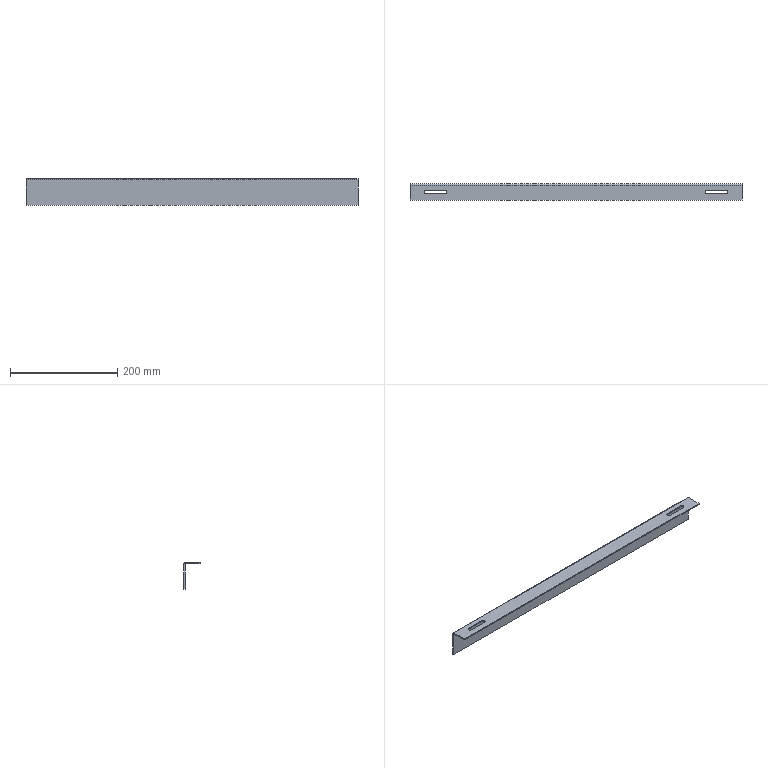Part | STEP file | FHD-021-010 L-shaped support rail | 1 solid | 18 faces | box 620 x 30 x 50 mm | volume 94894 mm3 | plane 12 | cylinder 6 | commonest cylinder face diameters 7 x4 0.6 x1 4.6 x1
STEP:
#1=CARTESIAN_POINT('',(0.,0.,0.));
#2=DIRECTION('',(0.,0.,1.));
#3=DIRECTION('',(1.,0.,0.));
#4=AXIS2_PLACEMENT_3D('',#1,#2,#3);
#5=CARTESIAN_POINT('',(-310.,13.,-2.3));
#6=VERTEX_POINT('',#5);
#7=CARTESIAN_POINT('',(-310.,13.,-50.));
#8=VERTEX_POINT('',#7);
#9=CARTESIAN_POINT('',(-310.,13.,0.));
#10=DIRECTION('',(0.,0.,-1.));
#11=VECTOR('',#10,1.);
#12=LINE('',#9,#11);
#13=CARTESIAN_POINT('',(0.,13.,0.));
#14=DIRECTION('',(0.,-1.,0.));
#15=DIRECTION('',(0.,0.,-1.));
#16=AXIS2_PLACEMENT_3D('',#13,#14,#15);
#17=PLANE('',#16);
#18=CARTESIAN_POINT('',(0.,-310.));
#19=DIRECTION('',(1.,0.));
#20=VECTOR('',#19,1.);
#21=LINE('',#18,#20);
#22=(GEOMETRIC_REPRESENTATION_CONTEXT(2)PARAMETRIC_REPRESENTATION_CONTEXT()REPRESENTATION_CONTEXT('',''));
#23=DEFINITIONAL_REPRESENTATION('',(#21),#22);
#24=PCURVE('',#17,#23);
#25=CARTESIAN_POINT('',(-310.,15.,-2.));
#26=DIRECTION('',(1.,0.,0.));
#27=DIRECTION('',(0.,0.,-1.));
#28=AXIS2_PLACEMENT_3D('',#25,#26,#27);
#29=PLANE('',#28);
#30=CARTESIAN_POINT('',(-2.,-2.));
#31=DIRECTION('',(1.,0.));
#32=VECTOR('',#31,1.);
#33=LINE('',#30,#32);
#34=(GEOMETRIC_REPRESENTATION_CONTEXT(2)PARAMETRIC_REPRESENTATION_CONTEXT()REPRESENTATION_CONTEXT('',''));
#35=DEFINITIONAL_REPRESENTATION('',(#33),#34);
#36=PCURVE('',#29,#35);
#37=SURFACE_CURVE('',#12,(#24,#36),.PCURVE_S1.);
#38=EDGE_CURVE('',#6,#8,#37,.T.);
#39=ORIENTED_EDGE('',*,*,#38,.T.);
#40=CARTESIAN_POINT('',(310.,13.,-50.));
#41=VERTEX_POINT('',#40);
#42=CARTESIAN_POINT('',(0.,13.,-50.));
#43=DIRECTION('',(1.,0.,0.));
#44=VECTOR('',#43,1.);
#45=LINE('',#42,#44);
#46=CARTESIAN_POINT('',(50.,0.));
#47=DIRECTION('',(0.,1.));
#48=VECTOR('',#47,1.);
#49=LINE('',#46,#48);
#50=(GEOMETRIC_REPRESENTATION_CONTEXT(2)PARAMETRIC_REPRESENTATION_CONTEXT()REPRESENTATION_CONTEXT('',''));
#51=DEFINITIONAL_REPRESENTATION('',(#49),#50);
#52=PCURVE('',#17,#51);
#53=CARTESIAN_POINT('',(-310.,15.,-50.));
#54=DIRECTION('',(0.,0.,1.));
#55=DIRECTION('',(0.,-1.,0.));
#56=AXIS2_PLACEMENT_3D('',#53,#54,#55);
#57=PLANE('',#56);
#58=CARTESIAN_POINT('',(2.,310.));
#59=DIRECTION('',(0.,1.));
#60=VECTOR('',#59,1.);
#61=LINE('',#58,#60);
#62=(GEOMETRIC_REPRESENTATION_CONTEXT(2)PARAMETRIC_REPRESENTATION_CONTEXT()REPRESENTATION_CONTEXT('',''));
#63=DEFINITIONAL_REPRESENTATION('',(#61),#62);
#64=PCURVE('',#57,#63);
#65=SURFACE_CURVE('',#45,(#52,#64),.PCURVE_S1.);
#66=EDGE_CURVE('',#8,#41,#65,.T.);
#67=ORIENTED_EDGE('',*,*,#66,.T.);
#68=CARTESIAN_POINT('',(310.,13.,-2.3));
#69=VERTEX_POINT('',#68);
#70=CARTESIAN_POINT('',(310.,13.,0.));
#71=DIRECTION('',(0.,0.,1.));
#72=VECTOR('',#71,1.);
#73=LINE('',#70,#72);
#74=CARTESIAN_POINT('',(0.,310.));
#75=DIRECTION('',(-1.,0.));
#76=VECTOR('',#75,1.);
#77=LINE('',#74,#76);
#78=(GEOMETRIC_REPRESENTATION_CONTEXT(2)PARAMETRIC_REPRESENTATION_CONTEXT()REPRESENTATION_CONTEXT('',''));
#79=DEFINITIONAL_REPRESENTATION('',(#77),#78);
#80=PCURVE('',#17,#79);
#81=CARTESIAN_POINT('',(310.,15.,-50.));
#82=DIRECTION('',(-1.,0.,0.));
#83=DIRECTION('',(0.,0.,1.));
#84=AXIS2_PLACEMENT_3D('',#81,#82,#83);
#85=PLANE('',#84);
#86=CARTESIAN_POINT('',(50.,-2.));
#87=DIRECTION('',(1.,0.));
#88=VECTOR('',#87,1.);
#89=LINE('',#86,#88);
#90=(GEOMETRIC_REPRESENTATION_CONTEXT(2)PARAMETRIC_REPRESENTATION_CONTEXT()REPRESENTATION_CONTEXT('',''));
#91=DEFINITIONAL_REPRESENTATION('',(#89),#90);
#92=PCURVE('',#85,#91);
#93=SURFACE_CURVE('',#73,(#80,#92),.PCURVE_S1.);
#94=EDGE_CURVE('',#41,#69,#93,.T.);
#95=ORIENTED_EDGE('',*,*,#94,.T.);
#96=CARTESIAN_POINT('',(0.,13.,-2.3));
#97=DIRECTION('',(-1.,0.,0.));
#98=VECTOR('',#97,1.);
#99=LINE('',#96,#98);
#100=CARTESIAN_POINT('',(2.3,0.));
#101=DIRECTION('',(0.,-1.));
#102=VECTOR('',#101,1.);
#103=LINE('',#100,#102);
#104=(GEOMETRIC_REPRESENTATION_CONTEXT(2)PARAMETRIC_REPRESENTATION_CONTEXT()REPRESENTATION_CONTEXT('',''));
#105=DEFINITIONAL_REPRESENTATION('',(#103),#104);
#106=PCURVE('',#17,#105);
#107=CARTESIAN_POINT('',(310.,12.7,-2.3));
#108=DIRECTION('',(1.,0.,0.));
#109=DIRECTION('',(0.,0.,-1.));
#110=AXIS2_PLACEMENT_3D('',#107,#108,#109);
#111=CYLINDRICAL_SURFACE('',#110,0.3);
#112=CARTESIAN_POINT('',(1.571,-310.));
#113=DIRECTION('',(0.,-1.));
#114=VECTOR('',#113,1.);
#115=LINE('',#112,#114);
#116=(GEOMETRIC_REPRESENTATION_CONTEXT(2)PARAMETRIC_REPRESENTATION_CONTEXT()REPRESENTATION_CONTEXT('',''));
#117=DEFINITIONAL_REPRESENTATION('',(#115),#116);
#118=PCURVE('',#111,#117);
#119=SURFACE_CURVE('',#99,(#106,#118),.PCURVE_S1.);
#120=EDGE_CURVE('',#69,#6,#119,.T.);
#121=ORIENTED_EDGE('',*,*,#120,.T.);
#122=EDGE_LOOP('',(#39,#67,#95,#121));
#123=FACE_BOUND('',#122,.T.);
#124=ADVANCED_FACE('',(#123),#17,.T.);
#125=CARTESIAN_POINT('',(-310.,15.,-50.));
#126=VERTEX_POINT('',#125);
#127=CARTESIAN_POINT('',(-310.,15.,-50.));
#128=DIRECTION('',(0.,-1.,0.));
#129=VECTOR('',#128,1.);
#130=LINE('',#127,#129);
#131=CARTESIAN_POINT('',(0.,0.));
#132=DIRECTION('',(1.,0.));
#133=VECTOR('',#132,1.);
#134=LINE('',#131,#133);
#135=(GEOMETRIC_REPRESENTATION_CONTEXT(2)PARAMETRIC_REPRESENTATION_CONTEXT()REPRESENTATION_CONTEXT('',''));
#136=DEFINITIONAL_REPRESENTATION('',(#134),#135);
#137=PCURVE('',#57,#136);
#138=CARTESIAN_POINT('',(48.,0.));
#139=DIRECTION('',(0.,-1.));
#140=VECTOR('',#139,1.);
#141=LINE('',#138,#140);
#142=(GEOMETRIC_REPRESENTATION_CONTEXT(2)PARAMETRIC_REPRESENTATION_CONTEXT()REPRESENTATION_CONTEXT('',''));
#143=DEFINITIONAL_REPRESENTATION('',(#141),#142);
#144=PCURVE('',#29,#143);
#145=SURFACE_CURVE('',#130,(#137,#144),.PCURVE_S1.);
#146=EDGE_CURVE('',#126,#8,#145,.T.);
#147=ORIENTED_EDGE('',*,*,#146,.F.);
#148=CARTESIAN_POINT('',(310.,15.,-50.));
#149=VERTEX_POINT('',#148);
#150=CARTESIAN_POINT('',(-310.,15.,-50.));
#151=DIRECTION('',(-1.,0.,0.));
#152=VECTOR('',#151,1.);
#153=LINE('',#150,#152);
#154=CARTESIAN_POINT('',(0.,0.));
#155=DIRECTION('',(0.,-1.));
#156=VECTOR('',#155,1.);
#157=LINE('',#154,#156);
#158=(GEOMETRIC_REPRESENTATION_CONTEXT(2)PARAMETRIC_REPRESENTATION_CONTEXT()REPRESENTATION_CONTEXT('',''));
#159=DEFINITIONAL_REPRESENTATION('',(#157),#158);
#160=PCURVE('',#57,#159);
#161=CARTESIAN_POINT('',(0.,15.,0.));
#162=DIRECTION('',(0.,-1.,0.));
#163=DIRECTION('',(0.,0.,-1.));
#164=AXIS2_PLACEMENT_3D('',#161,#162,#163);
#165=PLANE('',#164);
#166=CARTESIAN_POINT('',(50.,-310.));
#167=DIRECTION('',(0.,-1.));
#168=VECTOR('',#167,1.);
#169=LINE('',#166,#168);
#170=(GEOMETRIC_REPRESENTATION_CONTEXT(2)PARAMETRIC_REPRESENTATION_CONTEXT()REPRESENTATION_CONTEXT('',''));
#171=DEFINITIONAL_REPRESENTATION('',(#169),#170);
#172=PCURVE('',#165,#171);
#173=SURFACE_CURVE('',#153,(#160,#172),.PCURVE_S1.);
#174=EDGE_CURVE('',#149,#126,#173,.T.);
#175=ORIENTED_EDGE('',*,*,#174,.F.);
#176=CARTESIAN_POINT('',(310.,15.,-50.));
#177=DIRECTION('',(0.,1.,0.));
#178=VECTOR('',#177,1.);
#179=LINE('',#176,#178);
#180=CARTESIAN_POINT('',(0.,620.));
#181=DIRECTION('',(-1.,0.));
#182=VECTOR('',#181,1.);
#183=LINE('',#180,#182);
#184=(GEOMETRIC_REPRESENTATION_CONTEXT(2)PARAMETRIC_REPRESENTATION_CONTEXT()REPRESENTATION_CONTEXT('',''));
#185=DEFINITIONAL_REPRESENTATION('',(#183),#184);
#186=PCURVE('',#57,#185);
#187=CARTESIAN_POINT('',(0.,0.));
#188=DIRECTION('',(0.,1.));
#189=VECTOR('',#188,1.);
#190=LINE('',#187,#189);
#191=(GEOMETRIC_REPRESENTATION_CONTEXT(2)PARAMETRIC_REPRESENTATION_CONTEXT()REPRESENTATION_CONTEXT('',''));
#192=DEFINITIONAL_REPRESENTATION('',(#190),#191);
#193=PCURVE('',#85,#192);
#194=SURFACE_CURVE('',#179,(#186,#193),.PCURVE_S1.);
#195=EDGE_CURVE('',#41,#149,#194,.T.);
#196=ORIENTED_EDGE('',*,*,#195,.F.);
#197=ORIENTED_EDGE('',*,*,#66,.F.);
#198=EDGE_LOOP('',(#147,#175,#196,#197));
#199=FACE_BOUND('',#198,.T.);
#200=ADVANCED_FACE('',(#199),#57,.F.);
#201=CARTESIAN_POINT('',(-310.,15.,-2.3));
#202=VERTEX_POINT('',#201);
#203=CARTESIAN_POINT('',(-310.,15.,-2.));
#204=DIRECTION('',(0.,0.,1.));
#205=VECTOR('',#204,1.);
#206=LINE('',#203,#205);
#207=CARTESIAN_POINT('',(0.,0.));
#208=DIRECTION('',(-1.,0.));
#209=VECTOR('',#208,1.);
#210=LINE('',#207,#209);
#211=(GEOMETRIC_REPRESENTATION_CONTEXT(2)PARAMETRIC_REPRESENTATION_CONTEXT()REPRESENTATION_CONTEXT('',''));
#212=DEFINITIONAL_REPRESENTATION('',(#210),#211);
#213=PCURVE('',#29,#212);
#214=CARTESIAN_POINT('',(2.,-310.));
#215=DIRECTION('',(-1.,0.));
#216=VECTOR('',#215,1.);
#217=LINE('',#214,#216);
#218=(GEOMETRIC_REPRESENTATION_CONTEXT(2)PARAMETRIC_REPRESENTATION_CONTEXT()REPRESENTATION_CONTEXT('',''));
#219=DEFINITIONAL_REPRESENTATION('',(#217),#218);
#220=PCURVE('',#165,#219);
#221=SURFACE_CURVE('',#206,(#213,#220),.PCURVE_S1.);
#222=EDGE_CURVE('',#126,#202,#221,.T.);
#223=ORIENTED_EDGE('',*,*,#222,.F.);
#224=ORIENTED_EDGE('',*,*,#146,.T.);
#225=ORIENTED_EDGE('',*,*,#38,.F.);
#226=CARTESIAN_POINT('',(-310.,12.7,-2.));
#227=VERTEX_POINT('',#226);
#228=CARTESIAN_POINT('',(-310.,12.7,-2.3));
#229=DIRECTION('',(1.,0.,0.));
#230=DIRECTION('',(0.,0.,-1.));
#231=AXIS2_PLACEMENT_3D('',#228,#229,#230);
#232=CIRCLE('',#231,0.3);
#233=CARTESIAN_POINT('',(0.3,-2.3));
#234=DIRECTION('',(1.,0.));
#235=AXIS2_PLACEMENT_2D('',#233,#234);
#236=CIRCLE('',#235,0.3);
#237=(GEOMETRIC_REPRESENTATION_CONTEXT(2)PARAMETRIC_REPRESENTATION_CONTEXT()REPRESENTATION_CONTEXT('',''));
#238=DEFINITIONAL_REPRESENTATION('',(#236),#237);
#239=PCURVE('',#29,#238);
#240=CARTESIAN_POINT('',(0.,-620.));
#241=DIRECTION('',(1.,0.));
#242=VECTOR('',#241,1.);
#243=LINE('',#240,#242);
#244=(GEOMETRIC_REPRESENTATION_CONTEXT(2)PARAMETRIC_REPRESENTATION_CONTEXT()REPRESENTATION_CONTEXT('',''));
#245=DEFINITIONAL_REPRESENTATION('',(#243),#244);
#246=PCURVE('',#111,#245);
#247=SURFACE_CURVE('',#232,(#239,#246),.PCURVE_S1.);
#248=EDGE_CURVE('',#6,#227,#247,.T.);
#249=ORIENTED_EDGE('',*,*,#248,.T.);
#250=CARTESIAN_POINT('',(-310.,-15.,-2.));
#251=VERTEX_POINT('',#250);
#252=CARTESIAN_POINT('',(-310.,0.,-2.));
#253=DIRECTION('',(0.,1.,0.));
#254=VECTOR('',#253,1.);
#255=LINE('',#252,#254);
#256=CARTESIAN_POINT('',(0.,-15.));
#257=DIRECTION('',(0.,1.));
#258=VECTOR('',#257,1.);
#259=LINE('',#256,#258);
#260=(GEOMETRIC_REPRESENTATION_CONTEXT(2)PARAMETRIC_REPRESENTATION_CONTEXT()REPRESENTATION_CONTEXT('',''));
#261=DEFINITIONAL_REPRESENTATION('',(#259),#260);
#262=PCURVE('',#29,#261);
#263=CARTESIAN_POINT('',(0.,0.,-2.));
#264=DIRECTION('',(0.,0.,-1.));
#265=DIRECTION('',(-1.,0.,0.));
#266=AXIS2_PLACEMENT_3D('',#263,#264,#265);
#267=PLANE('',#266);
#268=CARTESIAN_POINT('',(310.,0.));
#269=DIRECTION('',(0.,1.));
#270=VECTOR('',#269,1.);
#271=LINE('',#268,#270);
#272=(GEOMETRIC_REPRESENTATION_CONTEXT(2)PARAMETRIC_REPRESENTATION_CONTEXT()REPRESENTATION_CONTEXT('',''));
#273=DEFINITIONAL_REPRESENTATION('',(#271),#272);
#274=PCURVE('',#267,#273);
#275=SURFACE_CURVE('',#255,(#262,#274),.PCURVE_S1.);
#276=EDGE_CURVE('',#251,#227,#275,.T.);
#277=ORIENTED_EDGE('',*,*,#276,.F.);
#278=CARTESIAN_POINT('',(-310.,-15.,0.));
#279=VERTEX_POINT('',#278);
#280=CARTESIAN_POINT('',(-310.,-15.,-2.));
#281=DIRECTION('',(0.,0.,1.));
#282=VECTOR('',#281,1.);
#283=LINE('',#280,#282);
#284=CARTESIAN_POINT('',(0.,-30.));
#285=DIRECTION('',(-1.,0.));
#286=VECTOR('',#285,1.);
#287=LINE('',#284,#286);
#288=(GEOMETRIC_REPRESENTATION_CONTEXT(2)PARAMETRIC_REPRESENTATION_CONTEXT()REPRESENTATION_CONTEXT('',''));
#289=DEFINITIONAL_REPRESENTATION('',(#287),#288);
#290=PCURVE('',#29,#289);
#291=CARTESIAN_POINT('',(-310.,-15.,-2.));
#292=DIRECTION('',(0.,-1.,0.));
#293=DIRECTION('',(0.,0.,-1.));
#294=AXIS2_PLACEMENT_3D('',#291,#292,#293);
#295=PLANE('',#294);
#296=CARTESIAN_POINT('',(0.,0.));
#297=DIRECTION('',(-1.,0.));
#298=VECTOR('',#297,1.);
#299=LINE('',#296,#298);
#300=(GEOMETRIC_REPRESENTATION_CONTEXT(2)PARAMETRIC_REPRESENTATION_CONTEXT()REPRESENTATION_CONTEXT('',''));
#301=DEFINITIONAL_REPRESENTATION('',(#299),#300);
#302=PCURVE('',#295,#301);
#303=SURFACE_CURVE('',#283,(#290,#302),.PCURVE_S1.);
#304=EDGE_CURVE('',#251,#279,#303,.T.);
#305=ORIENTED_EDGE('',*,*,#304,.T.);
#306=CARTESIAN_POINT('',(-310.,12.7,0.));
#307=VERTEX_POINT('',#306);
#308=CARTESIAN_POINT('',(-310.,-15.,0.));
#309=DIRECTION('',(0.,1.,0.));
#310=VECTOR('',#309,1.);
#311=LINE('',#308,#310);
#312=CARTESIAN_POINT('',(-2.,-30.));
#313=DIRECTION('',(0.,1.));
#314=VECTOR('',#313,1.);
#315=LINE('',#312,#314);
#316=(GEOMETRIC_REPRESENTATION_CONTEXT(2)PARAMETRIC_REPRESENTATION_CONTEXT()REPRESENTATION_CONTEXT('',''));
#317=DEFINITIONAL_REPRESENTATION('',(#315),#316);
#318=PCURVE('',#29,#317);
#319=CARTESIAN_POINT('',(0.,0.,0.));
#320=DIRECTION('',(0.,0.,-1.));
#321=DIRECTION('',(-1.,0.,0.));
#322=AXIS2_PLACEMENT_3D('',#319,#320,#321);
#323=PLANE('',#322);
#324=CARTESIAN_POINT('',(310.,-15.));
#325=DIRECTION('',(0.,1.));
#326=VECTOR('',#325,1.);
#327=LINE('',#324,#326);
#328=(GEOMETRIC_REPRESENTATION_CONTEXT(2)PARAMETRIC_REPRESENTATION_CONTEXT()REPRESENTATION_CONTEXT('',''));
#329=DEFINITIONAL_REPRESENTATION('',(#327),#328);
#330=PCURVE('',#323,#329);
#331=SURFACE_CURVE('',#311,(#318,#330),.PCURVE_S1.);
#332=EDGE_CURVE('',#279,#307,#331,.T.);
#333=ORIENTED_EDGE('',*,*,#332,.T.);
#334=CARTESIAN_POINT('',(-310.,12.7,-2.3));
#335=DIRECTION('',(-1.,0.,0.));
#336=DIRECTION('',(0.,0.,-1.));
#337=AXIS2_PLACEMENT_3D('',#334,#335,#336);
#338=CIRCLE('',#337,2.3);
#339=CARTESIAN_POINT('',(2.6,-2.3));
#340=CARTESIAN_POINT('',(2.6,-6.284));
#341=CARTESIAN_POINT('',(-0.85,-4.292));
#342=CARTESIAN_POINT('',(-4.3,-2.3));
#343=CARTESIAN_POINT('',(-0.85,-0.3081));
#344=CARTESIAN_POINT('',(2.6,1.684));
#345=CARTESIAN_POINT('',(2.6,-2.3));
#346=(BOUNDED_CURVE()B_SPLINE_CURVE(2,(#339,#340,#341,#342,#343,#344,#345),.UNSPECIFIED.,.T.,.F.)B_SPLINE_CURVE_WITH_KNOTS((1,2,2,2,2,1),(-2.094,0.,2.094,4.189,6.283,8.378),.UNSPECIFIED.)CURVE()GEOMETRIC_REPRESENTATION_ITEM()RATIONAL_B_SPLINE_CURVE((1.,0.5,1.,0.5,1.,0.5,1.))REPRESENTATION_ITEM(''));
#347=(GEOMETRIC_REPRESENTATION_CONTEXT(2)PARAMETRIC_REPRESENTATION_CONTEXT()REPRESENTATION_CONTEXT('',''));
#348=DEFINITIONAL_REPRESENTATION('',(#346),#347);
#349=PCURVE('',#29,#348);
#350=CARTESIAN_POINT('',(310.,12.7,-2.3));
#351=DIRECTION('',(1.,0.,0.));
#352=DIRECTION('',(0.,0.,-1.));
#353=AXIS2_PLACEMENT_3D('',#350,#351,#352);
#354=CYLINDRICAL_SURFACE('',#353,2.3);
#355=CARTESIAN_POINT('',(6.283,-620.));
#356=DIRECTION('',(-1.,0.));
#357=VECTOR('',#356,1.);
#358=LINE('',#355,#357);
#359=(GEOMETRIC_REPRESENTATION_CONTEXT(2)PARAMETRIC_REPRESENTATION_CONTEXT()REPRESENTATION_CONTEXT('',''));
#360=DEFINITIONAL_REPRESENTATION('',(#358),#359);
#361=PCURVE('',#354,#360);
#362=SURFACE_CURVE('',#338,(#349,#361),.PCURVE_S1.);
#363=EDGE_CURVE('',#307,#202,#362,.T.);
#364=ORIENTED_EDGE('',*,*,#363,.T.);
#365=EDGE_LOOP('',(#223,#224,#225,#249,#277,#305,#333,#364));
#366=FACE_BOUND('',#365,.T.);
#367=ADVANCED_FACE('',(#366),#29,.F.);
#368=CARTESIAN_POINT('',(310.,12.7,-2.));
#369=VERTEX_POINT('',#368);
#370=CARTESIAN_POINT('',(310.,12.7,-2.));
#371=DIRECTION('',(1.,0.,0.));
#372=VECTOR('',#371,1.);
#373=LINE('',#370,#372);
#374=CARTESIAN_POINT('',(3.142,0.));
#375=DIRECTION('',(0.,1.));
#376=VECTOR('',#375,1.);
#377=LINE('',#374,#376);
#378=(GEOMETRIC_REPRESENTATION_CONTEXT(2)PARAMETRIC_REPRESENTATION_CONTEXT()REPRESENTATION_CONTEXT('',''));
#379=DEFINITIONAL_REPRESENTATION('',(#377),#378);
#380=PCURVE('',#111,#379);
#381=CARTESIAN_POINT('',(-310.,12.7));
#382=DIRECTION('',(-1.,0.));
#383=VECTOR('',#382,1.);
#384=LINE('',#381,#383);
#385=(GEOMETRIC_REPRESENTATION_CONTEXT(2)PARAMETRIC_REPRESENTATION_CONTEXT()REPRESENTATION_CONTEXT('',''));
#386=DEFINITIONAL_REPRESENTATION('',(#384),#385);
#387=PCURVE('',#267,#386);
#388=SURFACE_CURVE('',#373,(#380,#387),.PCURVE_S1.);
#389=EDGE_CURVE('',#227,#369,#388,.T.);
#390=ORIENTED_EDGE('',*,*,#389,.T.);
#391=CARTESIAN_POINT('',(310.,12.7,-2.3));
#392=DIRECTION('',(1.,0.,0.));
#393=DIRECTION('',(0.,0.,-1.));
#394=AXIS2_PLACEMENT_3D('',#391,#392,#393);
#395=CIRCLE('',#394,0.3);
#396=CARTESIAN_POINT('',(0.,0.));
#397=DIRECTION('',(1.,0.));
#398=VECTOR('',#397,1.);
#399=LINE('',#396,#398);
#400=(GEOMETRIC_REPRESENTATION_CONTEXT(2)PARAMETRIC_REPRESENTATION_CONTEXT()REPRESENTATION_CONTEXT('',''));
#401=DEFINITIONAL_REPRESENTATION('',(#399),#400);
#402=PCURVE('',#111,#401);
#403=CARTESIAN_POINT('',(47.4,-2.3));
#404=CARTESIAN_POINT('',(47.4,-1.78));
#405=CARTESIAN_POINT('',(47.85,-2.04));
#406=CARTESIAN_POINT('',(48.3,-2.3));
#407=CARTESIAN_POINT('',(47.85,-2.56));
#408=CARTESIAN_POINT('',(47.4,-2.82));
#409=CARTESIAN_POINT('',(47.4,-2.3));
#410=(BOUNDED_CURVE()B_SPLINE_CURVE(2,(#403,#404,#405,#406,#407,#408,#409),.UNSPECIFIED.,.T.,.F.)B_SPLINE_CURVE_WITH_KNOTS((1,2,2,2,2,1),(-2.094,0.,2.094,4.189,6.283,8.378),.UNSPECIFIED.)CURVE()GEOMETRIC_REPRESENTATION_ITEM()RATIONAL_B_SPLINE_CURVE((1.,0.5,1.,0.5,1.,0.5,1.))REPRESENTATION_ITEM(''));
#411=(GEOMETRIC_REPRESENTATION_CONTEXT(2)PARAMETRIC_REPRESENTATION_CONTEXT()REPRESENTATION_CONTEXT('',''));
#412=DEFINITIONAL_REPRESENTATION('',(#410),#411);
#413=PCURVE('',#85,#412);
#414=SURFACE_CURVE('',#395,(#402,#413),.PCURVE_S1.);
#415=EDGE_CURVE('',#69,#369,#414,.T.);
#416=ORIENTED_EDGE('',*,*,#415,.F.);
#417=ORIENTED_EDGE('',*,*,#120,.T.);
#418=ORIENTED_EDGE('',*,*,#248,.T.);
#419=EDGE_LOOP('',(#390,#416,#417,#418));
#420=FACE_BOUND('',#419,.F.);
#421=ADVANCED_FACE('',(#420),#111,.F.);
#422=ORIENTED_EDGE('',*,*,#94,.F.);
#423=ORIENTED_EDGE('',*,*,#195,.T.);
#424=CARTESIAN_POINT('',(310.,15.,-2.3));
#425=VERTEX_POINT('',#424);
#426=CARTESIAN_POINT('',(310.,15.,-50.));
#427=DIRECTION('',(0.,0.,-1.));
#428=VECTOR('',#427,1.);
#429=LINE('',#426,#428);
#430=CARTESIAN_POINT('',(0.,0.));
#431=DIRECTION('',(-1.,0.));
#432=VECTOR('',#431,1.);
#433=LINE('',#430,#432);
#434=(GEOMETRIC_REPRESENTATION_CONTEXT(2)PARAMETRIC_REPRESENTATION_CONTEXT()REPRESENTATION_CONTEXT('',''));
#435=DEFINITIONAL_REPRESENTATION('',(#433),#434);
#436=PCURVE('',#85,#435);
#437=CARTESIAN_POINT('',(50.,310.));
#438=DIRECTION('',(1.,0.));
#439=VECTOR('',#438,1.);
#440=LINE('',#437,#439);
#441=(GEOMETRIC_REPRESENTATION_CONTEXT(2)PARAMETRIC_REPRESENTATION_CONTEXT()REPRESENTATION_CONTEXT('',''));
#442=DEFINITIONAL_REPRESENTATION('',(#440),#441);
#443=PCURVE('',#165,#442);
#444=SURFACE_CURVE('',#429,(#436,#443),.PCURVE_S1.);
#445=EDGE_CURVE('',#425,#149,#444,.T.);
#446=ORIENTED_EDGE('',*,*,#445,.F.);
#447=CARTESIAN_POINT('',(310.,12.7,0.));
#448=VERTEX_POINT('',#447);
#449=CARTESIAN_POINT('',(310.,12.7,-2.3));
#450=DIRECTION('',(-1.,0.,0.));
#451=DIRECTION('',(0.,0.,-1.));
#452=AXIS2_PLACEMENT_3D('',#449,#450,#451);
#453=CIRCLE('',#452,2.3);
#454=CARTESIAN_POINT('',(47.7,-2.3));
#455=DIRECTION('',(-1.,0.));
#456=AXIS2_PLACEMENT_2D('',#454,#455);
#457=CIRCLE('',#456,2.3);
#458=(GEOMETRIC_REPRESENTATION_CONTEXT(2)PARAMETRIC_REPRESENTATION_CONTEXT()REPRESENTATION_CONTEXT('',''));
#459=DEFINITIONAL_REPRESENTATION('',(#457),#458);
#460=PCURVE('',#85,#459);
#461=CARTESIAN_POINT('',(6.283,0.));
#462=DIRECTION('',(-1.,0.));
#463=VECTOR('',#462,1.);
#464=LINE('',#461,#463);
#465=(GEOMETRIC_REPRESENTATION_CONTEXT(2)PARAMETRIC_REPRESENTATION_CONTEXT()REPRESENTATION_CONTEXT('',''));
#466=DEFINITIONAL_REPRESENTATION('',(#464),#465);
#467=PCURVE('',#354,#466);
#468=SURFACE_CURVE('',#453,(#460,#467),.PCURVE_S1.);
#469=EDGE_CURVE('',#448,#425,#468,.T.);
#470=ORIENTED_EDGE('',*,*,#469,.F.);
#471=CARTESIAN_POINT('',(310.,-15.,0.));
#472=VERTEX_POINT('',#471);
#473=CARTESIAN_POINT('',(310.,-15.,0.));
#474=DIRECTION('',(0.,-1.,0.));
#475=VECTOR('',#474,1.);
#476=LINE('',#473,#475);
#477=CARTESIAN_POINT('',(50.,-30.));
#478=DIRECTION('',(0.,-1.));
#479=VECTOR('',#478,1.);
#480=LINE('',#477,#479);
#481=(GEOMETRIC_REPRESENTATION_CONTEXT(2)PARAMETRIC_REPRESENTATION_CONTEXT()REPRESENTATION_CONTEXT('',''));
#482=DEFINITIONAL_REPRESENTATION('',(#480),#481);
#483=PCURVE('',#85,#482);
#484=CARTESIAN_POINT('',(-310.,-15.));
#485=DIRECTION('',(0.,-1.));
#486=VECTOR('',#485,1.);
#487=LINE('',#484,#486);
#488=(GEOMETRIC_REPRESENTATION_CONTEXT(2)PARAMETRIC_REPRESENTATION_CONTEXT()REPRESENTATION_CONTEXT('',''));
#489=DEFINITIONAL_REPRESENTATION('',(#487),#488);
#490=PCURVE('',#323,#489);
#491=SURFACE_CURVE('',#476,(#483,#490),.PCURVE_S1.);
#492=EDGE_CURVE('',#448,#472,#491,.T.);
#493=ORIENTED_EDGE('',*,*,#492,.T.);
#494=CARTESIAN_POINT('',(310.,-15.,-2.));
#495=VERTEX_POINT('',#494);
#496=CARTESIAN_POINT('',(310.,-15.,-2.));
#497=DIRECTION('',(0.,0.,1.));
#498=VECTOR('',#497,1.);
#499=LINE('',#496,#498);
#500=CARTESIAN_POINT('',(48.,-30.));
#501=DIRECTION('',(1.,0.));
#502=VECTOR('',#501,1.);
#503=LINE('',#500,#502);
#504=(GEOMETRIC_REPRESENTATION_CONTEXT(2)PARAMETRIC_REPRESENTATION_CONTEXT()REPRESENTATION_CONTEXT('',''));
#505=DEFINITIONAL_REPRESENTATION('',(#503),#504);
#506=PCURVE('',#85,#505);
#507=CARTESIAN_POINT('',(0.,620.));
#508=DIRECTION('',(-1.,0.));
#509=VECTOR('',#508,1.);
#510=LINE('',#507,#509);
#511=(GEOMETRIC_REPRESENTATION_CONTEXT(2)PARAMETRIC_REPRESENTATION_CONTEXT()REPRESENTATION_CONTEXT('',''));
#512=DEFINITIONAL_REPRESENTATION('',(#510),#511);
#513=PCURVE('',#295,#512);
#514=SURFACE_CURVE('',#499,(#506,#513),.PCURVE_S1.);
#515=EDGE_CURVE('',#495,#472,#514,.T.);
#516=ORIENTED_EDGE('',*,*,#515,.F.);
#517=CARTESIAN_POINT('',(310.,0.,-2.));
#518=DIRECTION('',(0.,-1.,0.));
#519=VECTOR('',#518,1.);
#520=LINE('',#517,#519);
#521=CARTESIAN_POINT('',(48.,-15.));
#522=DIRECTION('',(0.,-1.));
#523=VECTOR('',#522,1.);
#524=LINE('',#521,#523);
#525=(GEOMETRIC_REPRESENTATION_CONTEXT(2)PARAMETRIC_REPRESENTATION_CONTEXT()REPRESENTATION_CONTEXT('',''));
#526=DEFINITIONAL_REPRESENTATION('',(#524),#525);
#527=PCURVE('',#85,#526);
#528=CARTESIAN_POINT('',(-310.,0.));
#529=DIRECTION('',(0.,-1.));
#530=VECTOR('',#529,1.);
#531=LINE('',#528,#530);
#532=(GEOMETRIC_REPRESENTATION_CONTEXT(2)PARAMETRIC_REPRESENTATION_CONTEXT()REPRESENTATION_CONTEXT('',''));
#533=DEFINITIONAL_REPRESENTATION('',(#531),#532);
#534=PCURVE('',#267,#533);
#535=SURFACE_CURVE('',#520,(#527,#534),.PCURVE_S1.);
#536=EDGE_CURVE('',#369,#495,#535,.T.);
#537=ORIENTED_EDGE('',*,*,#536,.F.);
#538=ORIENTED_EDGE('',*,*,#415,.F.);
#539=EDGE_LOOP('',(#422,#423,#446,#470,#493,#516,#537,#538));
#540=FACE_BOUND('',#539,.T.);
#541=ADVANCED_FACE('',(#540),#85,.F.);
#542=ORIENTED_EDGE('',*,*,#445,.T.);
#543=ORIENTED_EDGE('',*,*,#174,.T.);
#544=ORIENTED_EDGE('',*,*,#222,.T.);
#545=CARTESIAN_POINT('',(0.,15.,-2.3));
#546=DIRECTION('',(-1.,0.,0.));
#547=VECTOR('',#546,1.);
#548=LINE('',#545,#547);
#549=CARTESIAN_POINT('',(2.3,0.));
#550=DIRECTION('',(0.,-1.));
#551=VECTOR('',#550,1.);
#552=LINE('',#549,#551);
#553=(GEOMETRIC_REPRESENTATION_CONTEXT(2)PARAMETRIC_REPRESENTATION_CONTEXT()REPRESENTATION_CONTEXT('',''));
#554=DEFINITIONAL_REPRESENTATION('',(#552),#553);
#555=PCURVE('',#165,#554);
#556=CARTESIAN_POINT('',(1.571,-310.));
#557=DIRECTION('',(0.,-1.));
#558=VECTOR('',#557,1.);
#559=LINE('',#556,#558);
#560=(GEOMETRIC_REPRESENTATION_CONTEXT(2)PARAMETRIC_REPRESENTATION_CONTEXT()REPRESENTATION_CONTEXT('',''));
#561=DEFINITIONAL_REPRESENTATION('',(#559),#560);
#562=PCURVE('',#354,#561);
#563=SURFACE_CURVE('',#548,(#555,#562),.PCURVE_S1.);
#564=EDGE_CURVE('',#425,#202,#563,.T.);
#565=ORIENTED_EDGE('',*,*,#564,.F.);
#566=EDGE_LOOP('',(#542,#543,#544,#565));
#567=FACE_BOUND('',#566,.T.);
#568=ADVANCED_FACE('',(#567),#165,.F.);
#569=ORIENTED_EDGE('',*,*,#536,.T.);
#570=CARTESIAN_POINT('',(0.,-15.,-2.));
#571=DIRECTION('',(-1.,0.,0.));
#572=VECTOR('',#571,1.);
#573=LINE('',#570,#572);
#574=CARTESIAN_POINT('',(0.,-15.));
#575=DIRECTION('',(1.,0.));
#576=VECTOR('',#575,1.);
#577=LINE('',#574,#576);
#578=(GEOMETRIC_REPRESENTATION_CONTEXT(2)PARAMETRIC_REPRESENTATION_CONTEXT()REPRESENTATION_CONTEXT('',''));
#579=DEFINITIONAL_REPRESENTATION('',(#577),#578);
#580=PCURVE('',#267,#579);
#581=CARTESIAN_POINT('',(0.,310.));
#582=DIRECTION('',(0.,-1.));
#583=VECTOR('',#582,1.);
#584=LINE('',#581,#583);
#585=(GEOMETRIC_REPRESENTATION_CONTEXT(2)PARAMETRIC_REPRESENTATION_CONTEXT()REPRESENTATION_CONTEXT('',''));
#586=DEFINITIONAL_REPRESENTATION('',(#584),#585);
#587=PCURVE('',#295,#586);
#588=SURFACE_CURVE('',#573,(#580,#587),.PCURVE_S1.);
#589=EDGE_CURVE('',#495,#251,#588,.T.);
#590=ORIENTED_EDGE('',*,*,#589,.T.);
#591=ORIENTED_EDGE('',*,*,#276,.T.);
#592=ORIENTED_EDGE('',*,*,#389,.T.);
#593=EDGE_LOOP('',(#569,#590,#591,#592));
#594=FACE_BOUND('',#593,.T.);
#595=CARTESIAN_POINT('',(245.,3.5,-2.));
#596=VERTEX_POINT('',#595);
#597=CARTESIAN_POINT('',(245.,-3.5,-2.));
#598=VERTEX_POINT('',#597);
#599=CARTESIAN_POINT('',(245.,0.,-2.));
#600=DIRECTION('',(0.,0.,1.));
#601=DIRECTION('',(-1.,0.,0.));
#602=AXIS2_PLACEMENT_3D('',#599,#600,#601);
#603=CIRCLE('',#602,3.5);
#604=CARTESIAN_POINT('',(-241.5,0.));
#605=CARTESIAN_POINT('',(-241.5,-6.062));
#606=CARTESIAN_POINT('',(-246.75,-3.031));
#607=CARTESIAN_POINT('',(-252.,0.));
#608=CARTESIAN_POINT('',(-246.75,3.031));
#609=CARTESIAN_POINT('',(-241.5,6.062));
#610=CARTESIAN_POINT('',(-241.5,0.));
#611=(BOUNDED_CURVE()B_SPLINE_CURVE(2,(#604,#605,#606,#607,#608,#609,#610),.UNSPECIFIED.,.T.,.F.)B_SPLINE_CURVE_WITH_KNOTS((1,2,2,2,2,1),(-2.094,0.,2.094,4.189,6.283,8.378),.UNSPECIFIED.)CURVE()GEOMETRIC_REPRESENTATION_ITEM()RATIONAL_B_SPLINE_CURVE((1.,0.5,1.,0.5,1.,0.5,1.))REPRESENTATION_ITEM(''));
#612=(GEOMETRIC_REPRESENTATION_CONTEXT(2)PARAMETRIC_REPRESENTATION_CONTEXT()REPRESENTATION_CONTEXT('',''));
#613=DEFINITIONAL_REPRESENTATION('',(#611),#612);
#614=PCURVE('',#267,#613);
#615=CARTESIAN_POINT('',(245.,0.,0.));
#616=DIRECTION('',(0.,0.,-1.));
#617=DIRECTION('',(-1.,0.,0.));
#618=AXIS2_PLACEMENT_3D('',#615,#616,#617);
#619=CYLINDRICAL_SURFACE('',#618,3.5);
#620=CARTESIAN_POINT('',(6.283,2.));
#621=DIRECTION('',(-1.,0.));
#622=VECTOR('',#621,1.);
#623=LINE('',#620,#622);
#624=(GEOMETRIC_REPRESENTATION_CONTEXT(2)PARAMETRIC_REPRESENTATION_CONTEXT()REPRESENTATION_CONTEXT('',''));
#625=DEFINITIONAL_REPRESENTATION('',(#623),#624);
#626=PCURVE('',#619,#625);
#627=SURFACE_CURVE('',#603,(#614,#626),.PCURVE_S1.);
#628=EDGE_CURVE('',#596,#598,#627,.T.);
#629=ORIENTED_EDGE('',*,*,#628,.T.);
#630=CARTESIAN_POINT('',(280.,-3.5,-2.));
#631=VERTEX_POINT('',#630);
#632=CARTESIAN_POINT('',(0.,-3.5,-2.));
#633=DIRECTION('',(1.,0.,0.));
#634=VECTOR('',#633,1.);
#635=LINE('',#632,#634);
#636=CARTESIAN_POINT('',(0.,-3.5));
#637=DIRECTION('',(-1.,0.));
#638=VECTOR('',#637,1.);
#639=LINE('',#636,#638);
#640=(GEOMETRIC_REPRESENTATION_CONTEXT(2)PARAMETRIC_REPRESENTATION_CONTEXT()REPRESENTATION_CONTEXT('',''));
#641=DEFINITIONAL_REPRESENTATION('',(#639),#640);
#642=PCURVE('',#267,#641);
#643=CARTESIAN_POINT('',(280.,-3.5,0.));
#644=DIRECTION('',(0.,-1.,0.));
#645=DIRECTION('',(1.,0.,0.));
#646=AXIS2_PLACEMENT_3D('',#643,#644,#645);
#647=PLANE('',#646);
#648=CARTESIAN_POINT('',(-280.,-2.));
#649=DIRECTION('',(1.,0.));
#650=VECTOR('',#649,1.);
#651=LINE('',#648,#650);
#652=(GEOMETRIC_REPRESENTATION_CONTEXT(2)PARAMETRIC_REPRESENTATION_CONTEXT()REPRESENTATION_CONTEXT('',''));
#653=DEFINITIONAL_REPRESENTATION('',(#651),#652);
#654=PCURVE('',#647,#653);
#655=SURFACE_CURVE('',#635,(#642,#654),.PCURVE_S1.);
#656=EDGE_CURVE('',#598,#631,#655,.T.);
#657=ORIENTED_EDGE('',*,*,#656,.T.);
#658=CARTESIAN_POINT('',(280.,3.5,-2.));
#659=VERTEX_POINT('',#658);
#660=CARTESIAN_POINT('',(280.,0.,-2.));
#661=DIRECTION('',(0.,0.,1.));
#662=DIRECTION('',(-1.,0.,0.));
#663=AXIS2_PLACEMENT_3D('',#660,#661,#662);
#664=CIRCLE('',#663,3.5);
#665=CARTESIAN_POINT('',(-276.5,0.));
#666=CARTESIAN_POINT('',(-276.5,-6.062));
#667=CARTESIAN_POINT('',(-281.75,-3.031));
#668=CARTESIAN_POINT('',(-287.,0.));
#669=CARTESIAN_POINT('',(-281.75,3.031));
#670=CARTESIAN_POINT('',(-276.5,6.062));
#671=CARTESIAN_POINT('',(-276.5,0.));
#672=(BOUNDED_CURVE()B_SPLINE_CURVE(2,(#665,#666,#667,#668,#669,#670,#671),.UNSPECIFIED.,.T.,.F.)B_SPLINE_CURVE_WITH_KNOTS((1,2,2,2,2,1),(-2.094,0.,2.094,4.189,6.283,8.378),.UNSPECIFIED.)CURVE()GEOMETRIC_REPRESENTATION_ITEM()RATIONAL_B_SPLINE_CURVE((1.,0.5,1.,0.5,1.,0.5,1.))REPRESENTATION_ITEM(''));
#673=(GEOMETRIC_REPRESENTATION_CONTEXT(2)PARAMETRIC_REPRESENTATION_CONTEXT()REPRESENTATION_CONTEXT('',''));
#674=DEFINITIONAL_REPRESENTATION('',(#672),#673);
#675=PCURVE('',#267,#674);
#676=CARTESIAN_POINT('',(280.,0.,0.));
#677=DIRECTION('',(0.,0.,-1.));
#678=DIRECTION('',(-1.,0.,0.));
#679=AXIS2_PLACEMENT_3D('',#676,#677,#678);
#680=CYLINDRICAL_SURFACE('',#679,3.5);
#681=CARTESIAN_POINT('',(6.283,2.));
#682=DIRECTION('',(-1.,0.));
#683=VECTOR('',#682,1.);
#684=LINE('',#681,#683);
#685=(GEOMETRIC_REPRESENTATION_CONTEXT(2)PARAMETRIC_REPRESENTATION_CONTEXT()REPRESENTATION_CONTEXT('',''));
#686=DEFINITIONAL_REPRESENTATION('',(#684),#685);
#687=PCURVE('',#680,#686);
#688=SURFACE_CURVE('',#664,(#675,#687),.PCURVE_S1.);
#689=EDGE_CURVE('',#631,#659,#688,.T.);
#690=ORIENTED_EDGE('',*,*,#689,.T.);
#691=CARTESIAN_POINT('',(0.,3.5,-2.));
#692=DIRECTION('',(-1.,0.,0.));
#693=VECTOR('',#692,1.);
#694=LINE('',#691,#693);
#695=CARTESIAN_POINT('',(0.,3.5));
#696=DIRECTION('',(1.,0.));
#697=VECTOR('',#696,1.);
#698=LINE('',#695,#697);
#699=(GEOMETRIC_REPRESENTATION_CONTEXT(2)PARAMETRIC_REPRESENTATION_CONTEXT()REPRESENTATION_CONTEXT('',''));
#700=DEFINITIONAL_REPRESENTATION('',(#698),#699);
#701=PCURVE('',#267,#700);
#702=CARTESIAN_POINT('',(280.,3.5,0.));
#703=DIRECTION('',(0.,1.,0.));
#704=DIRECTION('',(-1.,0.,0.));
#705=AXIS2_PLACEMENT_3D('',#702,#703,#704);
#706=PLANE('',#705);
#707=CARTESIAN_POINT('',(280.,-2.));
#708=DIRECTION('',(1.,0.));
#709=VECTOR('',#708,1.);
#710=LINE('',#707,#709);
#711=(GEOMETRIC_REPRESENTATION_CONTEXT(2)PARAMETRIC_REPRESENTATION_CONTEXT()REPRESENTATION_CONTEXT('',''));
#712=DEFINITIONAL_REPRESENTATION('',(#710),#711);
#713=PCURVE('',#706,#712);
#714=SURFACE_CURVE('',#694,(#701,#713),.PCURVE_S1.);
#715=EDGE_CURVE('',#659,#596,#714,.T.);
#716=ORIENTED_EDGE('',*,*,#715,.T.);
#717=EDGE_LOOP('',(#629,#657,#690,#716));
#718=FACE_BOUND('',#717,.T.);
#719=CARTESIAN_POINT('',(-245.,3.5,-2.));
#720=VERTEX_POINT('',#719);
#721=CARTESIAN_POINT('',(-280.,3.5,-2.));
#722=VERTEX_POINT('',#721);
#723=CARTESIAN_POINT('',(0.,3.5,-2.));
#724=DIRECTION('',(-1.,0.,0.));
#725=VECTOR('',#724,1.);
#726=LINE('',#723,#725);
#727=CARTESIAN_POINT('',(0.,3.5));
#728=DIRECTION('',(1.,0.));
#729=VECTOR('',#728,1.);
#730=LINE('',#727,#729);
#731=(GEOMETRIC_REPRESENTATION_CONTEXT(2)PARAMETRIC_REPRESENTATION_CONTEXT()REPRESENTATION_CONTEXT('',''));
#732=DEFINITIONAL_REPRESENTATION('',(#730),#731);
#733=PCURVE('',#267,#732);
#734=CARTESIAN_POINT('',(-280.,3.5,0.));
#735=DIRECTION('',(0.,1.,0.));
#736=DIRECTION('',(-1.,0.,0.));
#737=AXIS2_PLACEMENT_3D('',#734,#735,#736);
#738=PLANE('',#737);
#739=CARTESIAN_POINT('',(-280.,-2.));
#740=DIRECTION('',(1.,0.));
#741=VECTOR('',#740,1.);
#742=LINE('',#739,#741);
#743=(GEOMETRIC_REPRESENTATION_CONTEXT(2)PARAMETRIC_REPRESENTATION_CONTEXT()REPRESENTATION_CONTEXT('',''));
#744=DEFINITIONAL_REPRESENTATION('',(#742),#743);
#745=PCURVE('',#738,#744);
#746=SURFACE_CURVE('',#726,(#733,#745),.PCURVE_S1.);
#747=EDGE_CURVE('',#720,#722,#746,.T.);
#748=ORIENTED_EDGE('',*,*,#747,.T.);
#749=CARTESIAN_POINT('',(-280.,-3.5,-2.));
#750=VERTEX_POINT('',#749);
#751=CARTESIAN_POINT('',(-280.,0.,-2.));
#752=DIRECTION('',(0.,0.,1.));
#753=DIRECTION('',(-1.,0.,0.));
#754=AXIS2_PLACEMENT_3D('',#751,#752,#753);
#755=CIRCLE('',#754,3.5);
#756=CARTESIAN_POINT('',(283.5,0.));
#757=CARTESIAN_POINT('',(283.5,-6.062));
#758=CARTESIAN_POINT('',(278.25,-3.031));
#759=CARTESIAN_POINT('',(273.,0.));
#760=CARTESIAN_POINT('',(278.25,3.031));
#761=CARTESIAN_POINT('',(283.5,6.062));
#762=CARTESIAN_POINT('',(283.5,0.));
#763=(BOUNDED_CURVE()B_SPLINE_CURVE(2,(#756,#757,#758,#759,#760,#761,#762),.UNSPECIFIED.,.T.,.F.)B_SPLINE_CURVE_WITH_KNOTS((1,2,2,2,2,1),(-2.094,0.,2.094,4.189,6.283,8.378),.UNSPECIFIED.)CURVE()GEOMETRIC_REPRESENTATION_ITEM()RATIONAL_B_SPLINE_CURVE((1.,0.5,1.,0.5,1.,0.5,1.))REPRESENTATION_ITEM(''));
#764=(GEOMETRIC_REPRESENTATION_CONTEXT(2)PARAMETRIC_REPRESENTATION_CONTEXT()REPRESENTATION_CONTEXT('',''));
#765=DEFINITIONAL_REPRESENTATION('',(#763),#764);
#766=PCURVE('',#267,#765);
#767=CARTESIAN_POINT('',(-280.,0.,0.));
#768=DIRECTION('',(0.,0.,-1.));
#769=DIRECTION('',(-1.,0.,0.));
#770=AXIS2_PLACEMENT_3D('',#767,#768,#769);
#771=CYLINDRICAL_SURFACE('',#770,3.5);
#772=CARTESIAN_POINT('',(6.283,2.));
#773=DIRECTION('',(-1.,0.));
#774=VECTOR('',#773,1.);
#775=LINE('',#772,#774);
#776=(GEOMETRIC_REPRESENTATION_CONTEXT(2)PARAMETRIC_REPRESENTATION_CONTEXT()REPRESENTATION_CONTEXT('',''));
#777=DEFINITIONAL_REPRESENTATION('',(#775),#776);
#778=PCURVE('',#771,#777);
#779=SURFACE_CURVE('',#755,(#766,#778),.PCURVE_S1.);
#780=EDGE_CURVE('',#722,#750,#779,.T.);
#781=ORIENTED_EDGE('',*,*,#780,.T.);
#782=CARTESIAN_POINT('',(-245.,-3.5,-2.));
#783=VERTEX_POINT('',#782);
#784=CARTESIAN_POINT('',(0.,-3.5,-2.));
#785=DIRECTION('',(1.,0.,0.));
#786=VECTOR('',#785,1.);
#787=LINE('',#784,#786);
#788=CARTESIAN_POINT('',(0.,-3.5));
#789=DIRECTION('',(-1.,0.));
#790=VECTOR('',#789,1.);
#791=LINE('',#788,#790);
#792=(GEOMETRIC_REPRESENTATION_CONTEXT(2)PARAMETRIC_REPRESENTATION_CONTEXT()REPRESENTATION_CONTEXT('',''));
#793=DEFINITIONAL_REPRESENTATION('',(#791),#792);
#794=PCURVE('',#267,#793);
#795=CARTESIAN_POINT('',(-280.,-3.5,0.));
#796=DIRECTION('',(0.,-1.,0.));
#797=DIRECTION('',(1.,0.,0.));
#798=AXIS2_PLACEMENT_3D('',#795,#796,#797);
#799=PLANE('',#798);
#800=CARTESIAN_POINT('',(280.,-2.));
#801=DIRECTION('',(1.,0.));
#802=VECTOR('',#801,1.);
#803=LINE('',#800,#802);
#804=(GEOMETRIC_REPRESENTATION_CONTEXT(2)PARAMETRIC_REPRESENTATION_CONTEXT()REPRESENTATION_CONTEXT('',''));
#805=DEFINITIONAL_REPRESENTATION('',(#803),#804);
#806=PCURVE('',#799,#805);
#807=SURFACE_CURVE('',#787,(#794,#806),.PCURVE_S1.);
#808=EDGE_CURVE('',#750,#783,#807,.T.);
#809=ORIENTED_EDGE('',*,*,#808,.T.);
#810=CARTESIAN_POINT('',(-245.,0.,-2.));
#811=DIRECTION('',(0.,0.,1.));
#812=DIRECTION('',(-1.,0.,0.));
#813=AXIS2_PLACEMENT_3D('',#810,#811,#812);
#814=CIRCLE('',#813,3.5);
#815=CARTESIAN_POINT('',(248.5,0.));
#816=CARTESIAN_POINT('',(248.5,-6.062));
#817=CARTESIAN_POINT('',(243.25,-3.031));
#818=CARTESIAN_POINT('',(238.,0.));
#819=CARTESIAN_POINT('',(243.25,3.031));
#820=CARTESIAN_POINT('',(248.5,6.062));
#821=CARTESIAN_POINT('',(248.5,0.));
#822=(BOUNDED_CURVE()B_SPLINE_CURVE(2,(#815,#816,#817,#818,#819,#820,#821),.UNSPECIFIED.,.T.,.F.)B_SPLINE_CURVE_WITH_KNOTS((1,2,2,2,2,1),(-2.094,0.,2.094,4.189,6.283,8.378),.UNSPECIFIED.)CURVE()GEOMETRIC_REPRESENTATION_ITEM()RATIONAL_B_SPLINE_CURVE((1.,0.5,1.,0.5,1.,0.5,1.))REPRESENTATION_ITEM(''));
#823=(GEOMETRIC_REPRESENTATION_CONTEXT(2)PARAMETRIC_REPRESENTATION_CONTEXT()REPRESENTATION_CONTEXT('',''));
#824=DEFINITIONAL_REPRESENTATION('',(#822),#823);
#825=PCURVE('',#267,#824);
#826=CARTESIAN_POINT('',(-245.,0.,0.));
#827=DIRECTION('',(0.,0.,-1.));
#828=DIRECTION('',(-1.,0.,0.));
#829=AXIS2_PLACEMENT_3D('',#826,#827,#828);
#830=CYLINDRICAL_SURFACE('',#829,3.5);
#831=CARTESIAN_POINT('',(6.283,2.));
#832=DIRECTION('',(-1.,0.));
#833=VECTOR('',#832,1.);
#834=LINE('',#831,#833);
#835=(GEOMETRIC_REPRESENTATION_CONTEXT(2)PARAMETRIC_REPRESENTATION_CONTEXT()REPRESENTATION_CONTEXT('',''));
#836=DEFINITIONAL_REPRESENTATION('',(#834),#835);
#837=PCURVE('',#830,#836);
#838=SURFACE_CURVE('',#814,(#825,#837),.PCURVE_S1.);
#839=EDGE_CURVE('',#783,#720,#838,.T.);
#840=ORIENTED_EDGE('',*,*,#839,.T.);
#841=EDGE_LOOP('',(#748,#781,#809,#840));
#842=FACE_BOUND('',#841,.T.);
#843=ADVANCED_FACE('',(#594,#718,#842),#267,.T.);
#844=ORIENTED_EDGE('',*,*,#564,.T.);
#845=ORIENTED_EDGE('',*,*,#363,.F.);
#846=CARTESIAN_POINT('',(310.,12.7,0.));
#847=DIRECTION('',(1.,0.,0.));
#848=VECTOR('',#847,1.);
#849=LINE('',#846,#848);
#850=CARTESIAN_POINT('',(3.142,0.));
#851=DIRECTION('',(0.,1.));
#852=VECTOR('',#851,1.);
#853=LINE('',#850,#852);
#854=(GEOMETRIC_REPRESENTATION_CONTEXT(2)PARAMETRIC_REPRESENTATION_CONTEXT()REPRESENTATION_CONTEXT('',''));
#855=DEFINITIONAL_REPRESENTATION('',(#853),#854);
#856=PCURVE('',#354,#855);
#857=CARTESIAN_POINT('',(-310.,12.7));
#858=DIRECTION('',(-1.,0.));
#859=VECTOR('',#858,1.);
#860=LINE('',#857,#859);
#861=(GEOMETRIC_REPRESENTATION_CONTEXT(2)PARAMETRIC_REPRESENTATION_CONTEXT()REPRESENTATION_CONTEXT('',''));
#862=DEFINITIONAL_REPRESENTATION('',(#860),#861);
#863=PCURVE('',#323,#862);
#864=SURFACE_CURVE('',#849,(#856,#863),.PCURVE_S1.);
#865=EDGE_CURVE('',#307,#448,#864,.T.);
#866=ORIENTED_EDGE('',*,*,#865,.T.);
#867=ORIENTED_EDGE('',*,*,#469,.T.);
#868=EDGE_LOOP('',(#844,#845,#866,#867));
#869=FACE_BOUND('',#868,.T.);
#870=ADVANCED_FACE('',(#869),#354,.T.);
#871=ORIENTED_EDGE('',*,*,#589,.F.);
#872=ORIENTED_EDGE('',*,*,#515,.T.);
#873=CARTESIAN_POINT('',(-310.,-15.,0.));
#874=DIRECTION('',(-1.,0.,0.));
#875=VECTOR('',#874,1.);
#876=LINE('',#873,#875);
#877=CARTESIAN_POINT('',(-2.,0.));
#878=DIRECTION('',(0.,-1.));
#879=VECTOR('',#878,1.);
#880=LINE('',#877,#879);
#881=(GEOMETRIC_REPRESENTATION_CONTEXT(2)PARAMETRIC_REPRESENTATION_CONTEXT()REPRESENTATION_CONTEXT('',''));
#882=DEFINITIONAL_REPRESENTATION('',(#880),#881);
#883=PCURVE('',#295,#882);
#884=CARTESIAN_POINT('',(310.,-15.));
#885=DIRECTION('',(1.,0.));
#886=VECTOR('',#885,1.);
#887=LINE('',#884,#886);
#888=(GEOMETRIC_REPRESENTATION_CONTEXT(2)PARAMETRIC_REPRESENTATION_CONTEXT()REPRESENTATION_CONTEXT('',''));
#889=DEFINITIONAL_REPRESENTATION('',(#887),#888);
#890=PCURVE('',#323,#889);
#891=SURFACE_CURVE('',#876,(#883,#890),.PCURVE_S1.);
#892=EDGE_CURVE('',#472,#279,#891,.T.);
#893=ORIENTED_EDGE('',*,*,#892,.T.);
#894=ORIENTED_EDGE('',*,*,#304,.F.);
#895=EDGE_LOOP('',(#871,#872,#893,#894));
#896=FACE_BOUND('',#895,.T.);
#897=ADVANCED_FACE('',(#896),#295,.T.);
#898=CARTESIAN_POINT('',(245.,-3.5,0.));
#899=VERTEX_POINT('',#898);
#900=CARTESIAN_POINT('',(245.,-3.5,0.));
#901=DIRECTION('',(0.,0.,-1.));
#902=VECTOR('',#901,1.);
#903=LINE('',#900,#902);
#904=CARTESIAN_POINT('',(-35.,0.));
#905=DIRECTION('',(0.,-1.));
#906=VECTOR('',#905,1.);
#907=LINE('',#904,#906);
#908=(GEOMETRIC_REPRESENTATION_CONTEXT(2)PARAMETRIC_REPRESENTATION_CONTEXT()REPRESENTATION_CONTEXT('',''));
#909=DEFINITIONAL_REPRESENTATION('',(#907),#908);
#910=PCURVE('',#647,#909);
#911=CARTESIAN_POINT('',(-1.571,0.));
#912=DIRECTION('',(0.,1.));
#913=VECTOR('',#912,1.);
#914=LINE('',#911,#913);
#915=(GEOMETRIC_REPRESENTATION_CONTEXT(2)PARAMETRIC_REPRESENTATION_CONTEXT()REPRESENTATION_CONTEXT('',''));
#916=DEFINITIONAL_REPRESENTATION('',(#914),#915);
#917=PCURVE('',#619,#916);
#918=SURFACE_CURVE('',#903,(#910,#917),.PCURVE_S1.);
#919=EDGE_CURVE('',#899,#598,#918,.T.);
#920=ORIENTED_EDGE('',*,*,#919,.F.);
#921=CARTESIAN_POINT('',(280.,-3.5,0.));
#922=VERTEX_POINT('',#921);
#923=CARTESIAN_POINT('',(280.,-3.5,0.));
#924=DIRECTION('',(-1.,0.,0.));
#925=VECTOR('',#924,1.);
#926=LINE('',#923,#925);
#927=CARTESIAN_POINT('',(0.,0.));
#928=DIRECTION('',(-1.,0.));
#929=VECTOR('',#928,1.);
#930=LINE('',#927,#929);
#931=(GEOMETRIC_REPRESENTATION_CONTEXT(2)PARAMETRIC_REPRESENTATION_CONTEXT()REPRESENTATION_CONTEXT('',''));
#932=DEFINITIONAL_REPRESENTATION('',(#930),#931);
#933=PCURVE('',#647,#932);
#934=CARTESIAN_POINT('',(-280.,-3.5));
#935=DIRECTION('',(1.,0.));
#936=VECTOR('',#935,1.);
#937=LINE('',#934,#936);
#938=(GEOMETRIC_REPRESENTATION_CONTEXT(2)PARAMETRIC_REPRESENTATION_CONTEXT()REPRESENTATION_CONTEXT('',''));
#939=DEFINITIONAL_REPRESENTATION('',(#937),#938);
#940=PCURVE('',#323,#939);
#941=SURFACE_CURVE('',#926,(#933,#940),.PCURVE_S1.);
#942=EDGE_CURVE('',#922,#899,#941,.T.);
#943=ORIENTED_EDGE('',*,*,#942,.F.);
#944=CARTESIAN_POINT('',(280.,-3.5,0.));
#945=DIRECTION('',(0.,0.,1.));
#946=VECTOR('',#945,1.);
#947=LINE('',#944,#946);
#948=CARTESIAN_POINT('',(0.,0.));
#949=DIRECTION('',(0.,1.));
#950=VECTOR('',#949,1.);
#951=LINE('',#948,#950);
#952=(GEOMETRIC_REPRESENTATION_CONTEXT(2)PARAMETRIC_REPRESENTATION_CONTEXT()REPRESENTATION_CONTEXT('',''));
#953=DEFINITIONAL_REPRESENTATION('',(#951),#952);
#954=PCURVE('',#647,#953);
#955=CARTESIAN_POINT('',(4.712,0.));
#956=DIRECTION('',(0.,-1.));
#957=VECTOR('',#956,1.);
#958=LINE('',#955,#957);
#959=(GEOMETRIC_REPRESENTATION_CONTEXT(2)PARAMETRIC_REPRESENTATION_CONTEXT()REPRESENTATION_CONTEXT('',''));
#960=DEFINITIONAL_REPRESENTATION('',(#958),#959);
#961=PCURVE('',#680,#960);
#962=SURFACE_CURVE('',#947,(#954,#961),.PCURVE_S1.);
#963=EDGE_CURVE('',#631,#922,#962,.T.);
#964=ORIENTED_EDGE('',*,*,#963,.F.);
#965=ORIENTED_EDGE('',*,*,#656,.F.);
#966=EDGE_LOOP('',(#920,#943,#964,#965));
#967=FACE_BOUND('',#966,.T.);
#968=ADVANCED_FACE('',(#967),#647,.F.);
#969=CARTESIAN_POINT('',(245.,3.5,0.));
#970=VERTEX_POINT('',#969);
#971=CARTESIAN_POINT('',(245.,3.5,0.));
#972=DIRECTION('',(0.,0.,-1.));
#973=VECTOR('',#972,1.);
#974=LINE('',#971,#973);
#975=CARTESIAN_POINT('',(1.571,0.));
#976=DIRECTION('',(0.,1.));
#977=VECTOR('',#976,1.);
#978=LINE('',#975,#977);
#979=(GEOMETRIC_REPRESENTATION_CONTEXT(2)PARAMETRIC_REPRESENTATION_CONTEXT()REPRESENTATION_CONTEXT('',''));
#980=DEFINITIONAL_REPRESENTATION('',(#978),#979);
#981=PCURVE('',#619,#980);
#982=CARTESIAN_POINT('',(35.,0.));
#983=DIRECTION('',(0.,-1.));
#984=VECTOR('',#983,1.);
#985=LINE('',#982,#984);
#986=(GEOMETRIC_REPRESENTATION_CONTEXT(2)PARAMETRIC_REPRESENTATION_CONTEXT()REPRESENTATION_CONTEXT('',''));
#987=DEFINITIONAL_REPRESENTATION('',(#985),#986);
#988=PCURVE('',#706,#987);
#989=SURFACE_CURVE('',#974,(#981,#988),.PCURVE_S1.);
#990=EDGE_CURVE('',#970,#596,#989,.T.);
#991=ORIENTED_EDGE('',*,*,#990,.T.);
#992=ORIENTED_EDGE('',*,*,#628,.T.);
#993=ORIENTED_EDGE('',*,*,#919,.F.);
#994=CARTESIAN_POINT('',(245.,0.,0.));
#995=DIRECTION('',(0.,0.,-1.));
#996=DIRECTION('',(-1.,0.,0.));
#997=AXIS2_PLACEMENT_3D('',#994,#995,#996);
#998=CIRCLE('',#997,3.5);
#999=CARTESIAN_POINT('',(-6.283,0.));
#1000=DIRECTION('',(1.,0.));
#1001=VECTOR('',#1000,1.);
#1002=LINE('',#999,#1001);
#1003=(GEOMETRIC_REPRESENTATION_CONTEXT(2)PARAMETRIC_REPRESENTATION_CONTEXT()REPRESENTATION_CONTEXT('',''));
#1004=DEFINITIONAL_REPRESENTATION('',(#1002),#1003);
#1005=PCURVE('',#619,#1004);
#1006=CARTESIAN_POINT('',(-245.,0.));
#1007=DIRECTION('',(1.,0.));
#1008=AXIS2_PLACEMENT_2D('',#1006,#1007);
#1009=CIRCLE('',#1008,3.5);
#1010=(GEOMETRIC_REPRESENTATION_CONTEXT(2)PARAMETRIC_REPRESENTATION_CONTEXT()REPRESENTATION_CONTEXT('',''));
#1011=DEFINITIONAL_REPRESENTATION('',(#1009),#1010);
#1012=PCURVE('',#323,#1011);
#1013=SURFACE_CURVE('',#998,(#1005,#1012),.PCURVE_S1.);
#1014=EDGE_CURVE('',#899,#970,#1013,.T.);
#1015=ORIENTED_EDGE('',*,*,#1014,.T.);
#1016=EDGE_LOOP('',(#991,#992,#993,#1015));
#1017=FACE_BOUND('',#1016,.F.);
#1018=ADVANCED_FACE('',(#1017),#619,.F.);
#1019=CARTESIAN_POINT('',(280.,3.5,0.));
#1020=VERTEX_POINT('',#1019);
#1021=CARTESIAN_POINT('',(280.,3.5,0.));
#1022=DIRECTION('',(0.,0.,-1.));
#1023=VECTOR('',#1022,1.);
#1024=LINE('',#1021,#1023);
#1025=CARTESIAN_POINT('',(0.,0.));
#1026=DIRECTION('',(0.,-1.));
#1027=VECTOR('',#1026,1.);
#1028=LINE('',#1025,#1027);
#1029=(GEOMETRIC_REPRESENTATION_CONTEXT(2)PARAMETRIC_REPRESENTATION_CONTEXT()REPRESENTATION_CONTEXT('',''));
#1030=DEFINITIONAL_REPRESENTATION('',(#1028),#1029);
#1031=PCURVE('',#706,#1030);
#1032=CARTESIAN_POINT('',(1.571,0.));
#1033=DIRECTION('',(0.,1.));
#1034=VECTOR('',#1033,1.);
#1035=LINE('',#1032,#1034);
#1036=(GEOMETRIC_REPRESENTATION_CONTEXT(2)PARAMETRIC_REPRESENTATION_CONTEXT()REPRESENTATION_CONTEXT('',''));
#1037=DEFINITIONAL_REPRESENTATION('',(#1035),#1036);
#1038=PCURVE('',#680,#1037);
#1039=SURFACE_CURVE('',#1024,(#1031,#1038),.PCURVE_S1.);
#1040=EDGE_CURVE('',#1020,#659,#1039,.T.);
#1041=ORIENTED_EDGE('',*,*,#1040,.F.);
#1042=CARTESIAN_POINT('',(280.,3.5,0.));
#1043=DIRECTION('',(1.,0.,0.));
#1044=VECTOR('',#1043,1.);
#1045=LINE('',#1042,#1044);
#1046=CARTESIAN_POINT('',(0.,0.));
#1047=DIRECTION('',(-1.,0.));
#1048=VECTOR('',#1047,1.);
#1049=LINE('',#1046,#1048);
#1050=(GEOMETRIC_REPRESENTATION_CONTEXT(2)PARAMETRIC_REPRESENTATION_CONTEXT()REPRESENTATION_CONTEXT('',''));
#1051=DEFINITIONAL_REPRESENTATION('',(#1049),#1050);
#1052=PCURVE('',#706,#1051);
#1053=CARTESIAN_POINT('',(-280.,3.5));
#1054=DIRECTION('',(-1.,0.));
#1055=VECTOR('',#1054,1.);
#1056=LINE('',#1053,#1055);
#1057=(GEOMETRIC_REPRESENTATION_CONTEXT(2)PARAMETRIC_REPRESENTATION_CONTEXT()REPRESENTATION_CONTEXT('',''));
#1058=DEFINITIONAL_REPRESENTATION('',(#1056),#1057);
#1059=PCURVE('',#323,#1058);
#1060=SURFACE_CURVE('',#1045,(#1052,#1059),.PCURVE_S1.);
#1061=EDGE_CURVE('',#970,#1020,#1060,.T.);
#1062=ORIENTED_EDGE('',*,*,#1061,.F.);
#1063=ORIENTED_EDGE('',*,*,#990,.T.);
#1064=ORIENTED_EDGE('',*,*,#715,.F.);
#1065=EDGE_LOOP('',(#1041,#1062,#1063,#1064));
#1066=FACE_BOUND('',#1065,.T.);
#1067=ADVANCED_FACE('',(#1066),#706,.F.);
#1068=ORIENTED_EDGE('',*,*,#689,.T.);
#1069=ORIENTED_EDGE('',*,*,#1040,.F.);
#1070=CARTESIAN_POINT('',(280.,0.,0.));
#1071=DIRECTION('',(0.,0.,-1.));
#1072=DIRECTION('',(-1.,0.,0.));
#1073=AXIS2_PLACEMENT_3D('',#1070,#1071,#1072);
#1074=CIRCLE('',#1073,3.5);
#1075=CARTESIAN_POINT('',(0.,0.));
#1076=DIRECTION('',(1.,0.));
#1077=VECTOR('',#1076,1.);
#1078=LINE('',#1075,#1077);
#1079=(GEOMETRIC_REPRESENTATION_CONTEXT(2)PARAMETRIC_REPRESENTATION_CONTEXT()REPRESENTATION_CONTEXT('',''));
#1080=DEFINITIONAL_REPRESENTATION('',(#1078),#1079);
#1081=PCURVE('',#680,#1080);
#1082=CARTESIAN_POINT('',(-280.,0.));
#1083=DIRECTION('',(1.,0.));
#1084=AXIS2_PLACEMENT_2D('',#1082,#1083);
#1085=CIRCLE('',#1084,3.5);
#1086=(GEOMETRIC_REPRESENTATION_CONTEXT(2)PARAMETRIC_REPRESENTATION_CONTEXT()REPRESENTATION_CONTEXT('',''));
#1087=DEFINITIONAL_REPRESENTATION('',(#1085),#1086);
#1088=PCURVE('',#323,#1087);
#1089=SURFACE_CURVE('',#1074,(#1081,#1088),.PCURVE_S1.);
#1090=EDGE_CURVE('',#1020,#922,#1089,.T.);
#1091=ORIENTED_EDGE('',*,*,#1090,.T.);
#1092=ORIENTED_EDGE('',*,*,#963,.F.);
#1093=EDGE_LOOP('',(#1068,#1069,#1091,#1092));
#1094=FACE_BOUND('',#1093,.F.);
#1095=ADVANCED_FACE('',(#1094),#680,.F.);
#1096=CARTESIAN_POINT('',(-280.,3.5,0.));
#1097=VERTEX_POINT('',#1096);
#1098=CARTESIAN_POINT('',(-280.,3.5,0.));
#1099=DIRECTION('',(0.,0.,-1.));
#1100=VECTOR('',#1099,1.);
#1101=LINE('',#1098,#1100);
#1102=CARTESIAN_POINT('',(1.571,0.));
#1103=DIRECTION('',(0.,1.));
#1104=VECTOR('',#1103,1.);
#1105=LINE('',#1102,#1104);
#1106=(GEOMETRIC_REPRESENTATION_CONTEXT(2)PARAMETRIC_REPRESENTATION_CONTEXT()REPRESENTATION_CONTEXT('',''));
#1107=DEFINITIONAL_REPRESENTATION('',(#1105),#1106);
#1108=PCURVE('',#771,#1107);
#1109=CARTESIAN_POINT('',(0.,0.));
#1110=DIRECTION('',(0.,-1.));
#1111=VECTOR('',#1110,1.);
#1112=LINE('',#1109,#1111);
#1113=(GEOMETRIC_REPRESENTATION_CONTEXT(2)PARAMETRIC_REPRESENTATION_CONTEXT()REPRESENTATION_CONTEXT('',''));
#1114=DEFINITIONAL_REPRESENTATION('',(#1112),#1113);
#1115=PCURVE('',#738,#1114);
#1116=SURFACE_CURVE('',#1101,(#1108,#1115),.PCURVE_S1.);
#1117=EDGE_CURVE('',#1097,#722,#1116,.T.);
#1118=ORIENTED_EDGE('',*,*,#1117,.T.);
#1119=ORIENTED_EDGE('',*,*,#780,.T.);
#1120=CARTESIAN_POINT('',(-280.,-3.5,0.));
#1121=VERTEX_POINT('',#1120);
#1122=CARTESIAN_POINT('',(-280.,-3.5,0.));
#1123=DIRECTION('',(0.,0.,-1.));
#1124=VECTOR('',#1123,1.);
#1125=LINE('',#1122,#1124);
#1126=CARTESIAN_POINT('',(-1.571,0.));
#1127=DIRECTION('',(0.,1.));
#1128=VECTOR('',#1127,1.);
#1129=LINE('',#1126,#1128);
#1130=(GEOMETRIC_REPRESENTATION_CONTEXT(2)PARAMETRIC_REPRESENTATION_CONTEXT()REPRESENTATION_CONTEXT('',''));
#1131=DEFINITIONAL_REPRESENTATION('',(#1129),#1130);
#1132=PCURVE('',#771,#1131);
#1133=CARTESIAN_POINT('',(0.,0.));
#1134=DIRECTION('',(0.,-1.));
#1135=VECTOR('',#1134,1.);
#1136=LINE('',#1133,#1135);
#1137=(GEOMETRIC_REPRESENTATION_CONTEXT(2)PARAMETRIC_REPRESENTATION_CONTEXT()REPRESENTATION_CONTEXT('',''));
#1138=DEFINITIONAL_REPRESENTATION('',(#1136),#1137);
#1139=PCURVE('',#799,#1138);
#1140=SURFACE_CURVE('',#1125,(#1132,#1139),.PCURVE_S1.);
#1141=EDGE_CURVE('',#1121,#750,#1140,.T.);
#1142=ORIENTED_EDGE('',*,*,#1141,.F.);
#1143=CARTESIAN_POINT('',(-280.,0.,0.));
#1144=DIRECTION('',(0.,0.,-1.));
#1145=DIRECTION('',(-1.,0.,0.));
#1146=AXIS2_PLACEMENT_3D('',#1143,#1144,#1145);
#1147=CIRCLE('',#1146,3.5);
#1148=CARTESIAN_POINT('',(-6.283,0.));
#1149=DIRECTION('',(1.,0.));
#1150=VECTOR('',#1149,1.);
#1151=LINE('',#1148,#1150);
#1152=(GEOMETRIC_REPRESENTATION_CONTEXT(2)PARAMETRIC_REPRESENTATION_CONTEXT()REPRESENTATION_CONTEXT('',''));
#1153=DEFINITIONAL_REPRESENTATION('',(#1151),#1152);
#1154=PCURVE('',#771,#1153);
#1155=CARTESIAN_POINT('',(280.,0.));
#1156=DIRECTION('',(1.,0.));
#1157=AXIS2_PLACEMENT_2D('',#1155,#1156);
#1158=CIRCLE('',#1157,3.5);
#1159=(GEOMETRIC_REPRESENTATION_CONTEXT(2)PARAMETRIC_REPRESENTATION_CONTEXT()REPRESENTATION_CONTEXT('',''));
#1160=DEFINITIONAL_REPRESENTATION('',(#1158),#1159);
#1161=PCURVE('',#323,#1160);
#1162=SURFACE_CURVE('',#1147,(#1154,#1161),.PCURVE_S1.);
#1163=EDGE_CURVE('',#1121,#1097,#1162,.T.);
#1164=ORIENTED_EDGE('',*,*,#1163,.T.);
#1165=EDGE_LOOP('',(#1118,#1119,#1142,#1164));
#1166=FACE_BOUND('',#1165,.F.);
#1167=ADVANCED_FACE('',(#1166),#771,.F.);
#1168=CARTESIAN_POINT('',(-245.,3.5,0.));
#1169=VERTEX_POINT('',#1168);
#1170=CARTESIAN_POINT('',(-245.,3.5,0.));
#1171=DIRECTION('',(0.,0.,-1.));
#1172=VECTOR('',#1171,1.);
#1173=LINE('',#1170,#1172);
#1174=CARTESIAN_POINT('',(-35.,0.));
#1175=DIRECTION('',(0.,-1.));
#1176=VECTOR('',#1175,1.);
#1177=LINE('',#1174,#1176);
#1178=(GEOMETRIC_REPRESENTATION_CONTEXT(2)PARAMETRIC_REPRESENTATION_CONTEXT()REPRESENTATION_CONTEXT('',''));
#1179=DEFINITIONAL_REPRESENTATION('',(#1177),#1178);
#1180=PCURVE('',#738,#1179);
#1181=CARTESIAN_POINT('',(1.571,0.));
#1182=DIRECTION('',(0.,1.));
#1183=VECTOR('',#1182,1.);
#1184=LINE('',#1181,#1183);
#1185=(GEOMETRIC_REPRESENTATION_CONTEXT(2)PARAMETRIC_REPRESENTATION_CONTEXT()REPRESENTATION_CONTEXT('',''));
#1186=DEFINITIONAL_REPRESENTATION('',(#1184),#1185);
#1187=PCURVE('',#830,#1186);
#1188=SURFACE_CURVE('',#1173,(#1180,#1187),.PCURVE_S1.);
#1189=EDGE_CURVE('',#1169,#720,#1188,.T.);
#1190=ORIENTED_EDGE('',*,*,#1189,.F.);
#1191=CARTESIAN_POINT('',(-280.,3.5,0.));
#1192=DIRECTION('',(1.,0.,0.));
#1193=VECTOR('',#1192,1.);
#1194=LINE('',#1191,#1193);
#1195=CARTESIAN_POINT('',(0.,0.));
#1196=DIRECTION('',(-1.,0.));
#1197=VECTOR('',#1196,1.);
#1198=LINE('',#1195,#1197);
#1199=(GEOMETRIC_REPRESENTATION_CONTEXT(2)PARAMETRIC_REPRESENTATION_CONTEXT()REPRESENTATION_CONTEXT('',''));
#1200=DEFINITIONAL_REPRESENTATION('',(#1198),#1199);
#1201=PCURVE('',#738,#1200);
#1202=CARTESIAN_POINT('',(280.,3.5));
#1203=DIRECTION('',(-1.,0.));
#1204=VECTOR('',#1203,1.);
#1205=LINE('',#1202,#1204);
#1206=(GEOMETRIC_REPRESENTATION_CONTEXT(2)PARAMETRIC_REPRESENTATION_CONTEXT()REPRESENTATION_CONTEXT('',''));
#1207=DEFINITIONAL_REPRESENTATION('',(#1205),#1206);
#1208=PCURVE('',#323,#1207);
#1209=SURFACE_CURVE('',#1194,(#1201,#1208),.PCURVE_S1.);
#1210=EDGE_CURVE('',#1097,#1169,#1209,.T.);
#1211=ORIENTED_EDGE('',*,*,#1210,.F.);
#1212=ORIENTED_EDGE('',*,*,#1117,.T.);
#1213=ORIENTED_EDGE('',*,*,#747,.F.);
#1214=EDGE_LOOP('',(#1190,#1211,#1212,#1213));
#1215=FACE_BOUND('',#1214,.T.);
#1216=ADVANCED_FACE('',(#1215),#738,.F.);
#1217=ORIENTED_EDGE('',*,*,#839,.T.);
#1218=ORIENTED_EDGE('',*,*,#1189,.F.);
#1219=CARTESIAN_POINT('',(-245.,-3.5,0.));
#1220=VERTEX_POINT('',#1219);
#1221=CARTESIAN_POINT('',(-245.,0.,0.));
#1222=DIRECTION('',(0.,0.,-1.));
#1223=DIRECTION('',(-1.,0.,0.));
#1224=AXIS2_PLACEMENT_3D('',#1221,#1222,#1223);
#1225=CIRCLE('',#1224,3.5);
#1226=CARTESIAN_POINT('',(0.,0.));
#1227=DIRECTION('',(1.,0.));
#1228=VECTOR('',#1227,1.);
#1229=LINE('',#1226,#1228);
#1230=(GEOMETRIC_REPRESENTATION_CONTEXT(2)PARAMETRIC_REPRESENTATION_CONTEXT()REPRESENTATION_CONTEXT('',''));
#1231=DEFINITIONAL_REPRESENTATION('',(#1229),#1230);
#1232=PCURVE('',#830,#1231);
#1233=CARTESIAN_POINT('',(245.,0.));
#1234=DIRECTION('',(1.,0.));
#1235=AXIS2_PLACEMENT_2D('',#1233,#1234);
#1236=CIRCLE('',#1235,3.5);
#1237=(GEOMETRIC_REPRESENTATION_CONTEXT(2)PARAMETRIC_REPRESENTATION_CONTEXT()REPRESENTATION_CONTEXT('',''));
#1238=DEFINITIONAL_REPRESENTATION('',(#1236),#1237);
#1239=PCURVE('',#323,#1238);
#1240=SURFACE_CURVE('',#1225,(#1232,#1239),.PCURVE_S1.);
#1241=EDGE_CURVE('',#1169,#1220,#1240,.T.);
#1242=ORIENTED_EDGE('',*,*,#1241,.T.);
#1243=CARTESIAN_POINT('',(-245.,-3.5,0.));
#1244=DIRECTION('',(0.,0.,-1.));
#1245=VECTOR('',#1244,1.);
#1246=LINE('',#1243,#1245);
#1247=CARTESIAN_POINT('',(4.712,0.));
#1248=DIRECTION('',(0.,1.));
#1249=VECTOR('',#1248,1.);
#1250=LINE('',#1247,#1249);
#1251=(GEOMETRIC_REPRESENTATION_CONTEXT(2)PARAMETRIC_REPRESENTATION_CONTEXT()REPRESENTATION_CONTEXT('',''));
#1252=DEFINITIONAL_REPRESENTATION('',(#1250),#1251);
#1253=PCURVE('',#830,#1252);
#1254=CARTESIAN_POINT('',(35.,0.));
#1255=DIRECTION('',(0.,-1.));
#1256=VECTOR('',#1255,1.);
#1257=LINE('',#1254,#1256);
#1258=(GEOMETRIC_REPRESENTATION_CONTEXT(2)PARAMETRIC_REPRESENTATION_CONTEXT()REPRESENTATION_CONTEXT('',''));
#1259=DEFINITIONAL_REPRESENTATION('',(#1257),#1258);
#1260=PCURVE('',#799,#1259);
#1261=SURFACE_CURVE('',#1246,(#1253,#1260),.PCURVE_S1.);
#1262=EDGE_CURVE('',#1220,#783,#1261,.T.);
#1263=ORIENTED_EDGE('',*,*,#1262,.T.);
#1264=EDGE_LOOP('',(#1217,#1218,#1242,#1263));
#1265=FACE_BOUND('',#1264,.F.);
#1266=ADVANCED_FACE('',(#1265),#830,.F.);
#1267=ORIENTED_EDGE('',*,*,#1141,.F.);
#1268=CARTESIAN_POINT('',(-280.,-3.5,0.));
#1269=DIRECTION('',(-1.,0.,0.));
#1270=VECTOR('',#1269,1.);
#1271=LINE('',#1268,#1270);
#1272=CARTESIAN_POINT('',(0.,0.));
#1273=DIRECTION('',(-1.,0.));
#1274=VECTOR('',#1273,1.);
#1275=LINE('',#1272,#1274);
#1276=(GEOMETRIC_REPRESENTATION_CONTEXT(2)PARAMETRIC_REPRESENTATION_CONTEXT()REPRESENTATION_CONTEXT('',''));
#1277=DEFINITIONAL_REPRESENTATION('',(#1275),#1276);
#1278=PCURVE('',#799,#1277);
#1279=CARTESIAN_POINT('',(280.,-3.5));
#1280=DIRECTION('',(1.,0.));
#1281=VECTOR('',#1280,1.);
#1282=LINE('',#1279,#1281);
#1283=(GEOMETRIC_REPRESENTATION_CONTEXT(2)PARAMETRIC_REPRESENTATION_CONTEXT()REPRESENTATION_CONTEXT('',''));
#1284=DEFINITIONAL_REPRESENTATION('',(#1282),#1283);
#1285=PCURVE('',#323,#1284);
#1286=SURFACE_CURVE('',#1271,(#1278,#1285),.PCURVE_S1.);
#1287=EDGE_CURVE('',#1220,#1121,#1286,.T.);
#1288=ORIENTED_EDGE('',*,*,#1287,.F.);
#1289=ORIENTED_EDGE('',*,*,#1262,.T.);
#1290=ORIENTED_EDGE('',*,*,#808,.F.);
#1291=EDGE_LOOP('',(#1267,#1288,#1289,#1290));
#1292=FACE_BOUND('',#1291,.T.);
#1293=ADVANCED_FACE('',(#1292),#799,.F.);
#1294=ORIENTED_EDGE('',*,*,#332,.F.);
#1295=ORIENTED_EDGE('',*,*,#892,.F.);
#1296=ORIENTED_EDGE('',*,*,#492,.F.);
#1297=ORIENTED_EDGE('',*,*,#865,.F.);
#1298=EDGE_LOOP('',(#1294,#1295,#1296,#1297));
#1299=FACE_BOUND('',#1298,.T.);
#1300=ORIENTED_EDGE('',*,*,#1090,.T.);
#1301=ORIENTED_EDGE('',*,*,#942,.T.);
#1302=ORIENTED_EDGE('',*,*,#1014,.T.);
#1303=ORIENTED_EDGE('',*,*,#1061,.T.);
#1304=EDGE_LOOP('',(#1300,#1301,#1302,#1303));
#1305=FACE_BOUND('',#1304,.T.);
#1306=ORIENTED_EDGE('',*,*,#1287,.T.);
#1307=ORIENTED_EDGE('',*,*,#1163,.T.);
#1308=ORIENTED_EDGE('',*,*,#1210,.T.);
#1309=ORIENTED_EDGE('',*,*,#1241,.T.);
#1310=EDGE_LOOP('',(#1306,#1307,#1308,#1309));
#1311=FACE_BOUND('',#1310,.T.);
#1312=ADVANCED_FACE('',(#1299,#1305,#1311),#323,.F.);
#1313=CLOSED_SHELL('',(#124,#200,#367,#421,#541,#568,#843,#870,#897,#968,#1018,#1067,#1095,#1167,#1216,#1266,#1293,#1312));
#1314=MANIFOLD_SOLID_BREP('',#1313);
#1315=(LENGTH_UNIT()NAMED_UNIT(*)SI_UNIT(.MILLI.,.METRE.));
#1316=UNCERTAINTY_MEASURE_WITH_UNIT(LENGTH_MEASURE(0.0000001),#1315,'','');
#1317=(NAMED_UNIT(*)PLANE_ANGLE_UNIT()SI_UNIT($,.RADIAN.));
#1318=(NAMED_UNIT(*)SI_UNIT($,.STERADIAN.)SOLID_ANGLE_UNIT());
#1319=(GEOMETRIC_REPRESENTATION_CONTEXT(3)GLOBAL_UNCERTAINTY_ASSIGNED_CONTEXT((#1316))GLOBAL_UNIT_ASSIGNED_CONTEXT((#1315,#1317,#1318))REPRESENTATION_CONTEXT('',''));
#1320=ADVANCED_BREP_SHAPE_REPRESENTATION('',(#4,#1314),#1319);